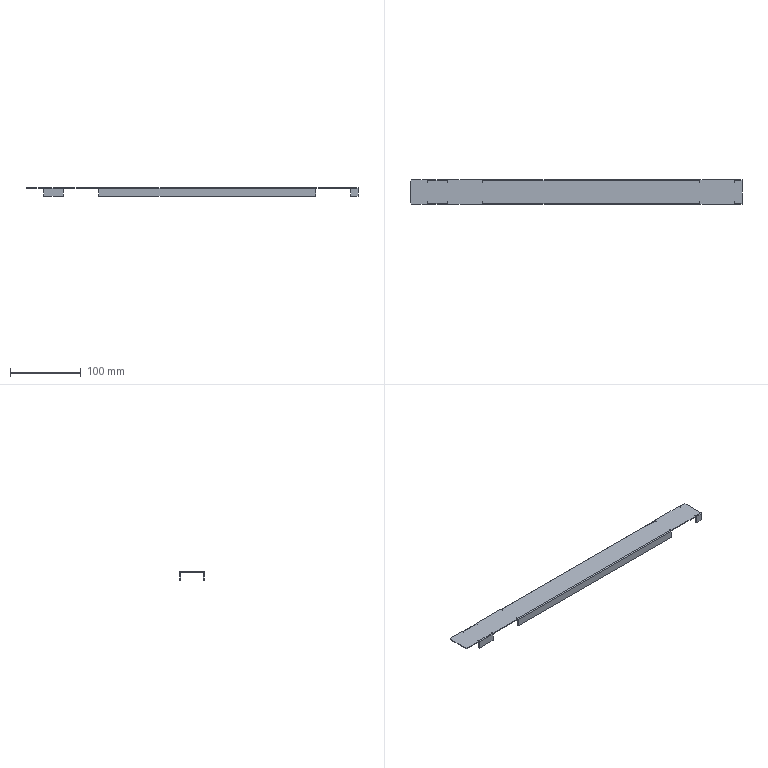Part | SolidWorks | features SMBaseFlange 2, Chamfer 1, Cut 1, EdgeFlange 1, FlatPattern 1, ICE 1, MirrorPattern 1, SheetMetal 1 | 1 solid | 96 faces | box 470 x 34 x 12 mm | volume 23344 mm3 | plane 84 | cylinder 12 | commonest cylinder face diameters 0.4 x6 2.4 x6